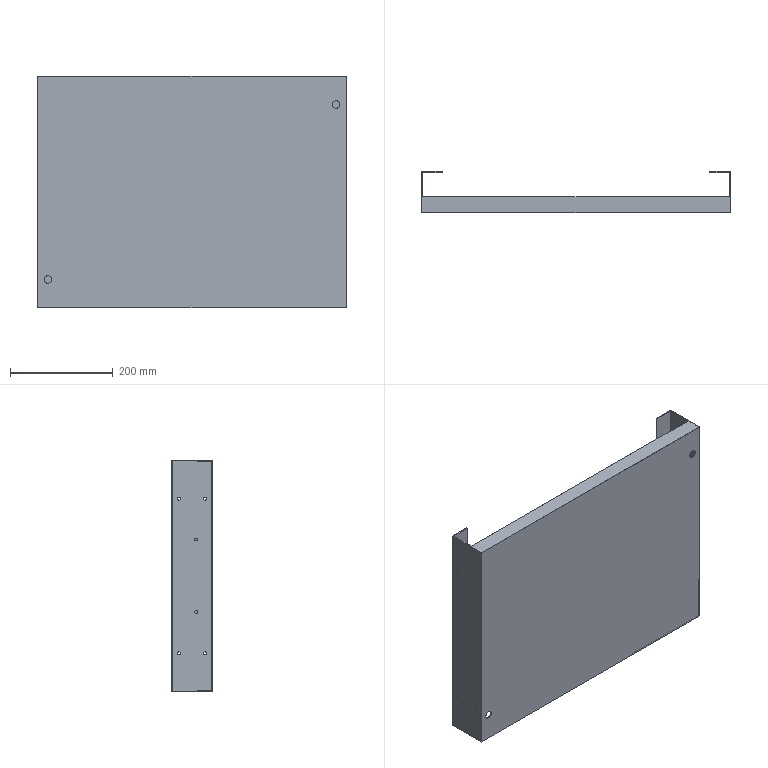Part | SolidWorks | features BaseBody 1 | 1 solid | 42 faces | box 600 x 80 x 450 mm | volume 814370 mm3 | cylinder 24 | plane 18 | commonest cylinder face diameters 5.5 x20 15 x4
STEP:
#1=CARTESIAN_POINT('',(301.946,-4083.973,1922.471));
#2=VERTEX_POINT('',#1);
#3=CARTESIAN_POINT('',(301.946,-4083.973,1907.471));
#4=VERTEX_POINT('',#3);
#5=CARTESIAN_POINT('',(301.946,-4083.973,1914.971));
#6=DIRECTION('',(0.,-1.,0.));
#7=DIRECTION('',(0.,0.,-1.));
#8=AXIS2_PLACEMENT_3D('',#5,#6,#7);
#9=CIRCLE('',#8,7.5);
#10=EDGE_CURVE('',#2,#4,#9,.T.);
#11=ORIENTED_EDGE('',*,*,#10,.F.);
#12=CARTESIAN_POINT('',(301.946,-4085.973,1922.471));
#13=VERTEX_POINT('',#12);
#14=CARTESIAN_POINT('',(301.946,-4104.978,1922.471));
#15=DIRECTION('',(0.,-1.,0.));
#16=VECTOR('',#15,1000.);
#17=LINE('',#14,#16);
#18=EDGE_CURVE('',#2,#13,#17,.T.);
#19=ORIENTED_EDGE('',*,*,#18,.T.);
#20=CARTESIAN_POINT('',(301.946,-4085.973,1907.471));
#21=VERTEX_POINT('',#20);
#22=CARTESIAN_POINT('',(301.946,-4085.973,1914.971));
#23=DIRECTION('',(0.,1.,0.));
#24=DIRECTION('',(0.,0.,-1.));
#25=AXIS2_PLACEMENT_3D('',#22,#23,#24);
#26=CIRCLE('',#25,7.5);
#27=EDGE_CURVE('',#21,#13,#26,.T.);
#28=ORIENTED_EDGE('',*,*,#27,.F.);
#29=CARTESIAN_POINT('',(301.946,-4104.978,1907.471));
#30=DIRECTION('',(0.,-1.,0.));
#31=VECTOR('',#30,1000.);
#32=LINE('',#29,#31);
#33=EDGE_CURVE('',#4,#21,#32,.T.);
#34=ORIENTED_EDGE('',*,*,#33,.F.);
#35=EDGE_LOOP('',(#11,#19,#28,#34));
#36=FACE_OUTER_BOUND('',#35,.T.);
#37=CARTESIAN_POINT('',(301.946,-4104.978,1914.971));
#38=DIRECTION('',(0.,-1.,0.));
#39=DIRECTION('',(0.,0.,-1.));
#40=AXIS2_PLACEMENT_3D('',#37,#38,#39);
#41=CYLINDRICAL_SURFACE('',#40,7.5);
#42=ADVANCED_FACE('',(#36),#41,.F.);
#43=CARTESIAN_POINT('',(861.946,-4083.973,2262.471));
#44=VERTEX_POINT('',#43);
#45=CARTESIAN_POINT('',(861.946,-4083.973,2247.471));
#46=VERTEX_POINT('',#45);
#47=CARTESIAN_POINT('',(861.946,-4083.973,2254.971));
#48=DIRECTION('',(0.,-1.,0.));
#49=DIRECTION('',(0.,0.,-1.));
#50=AXIS2_PLACEMENT_3D('',#47,#48,#49);
#51=CIRCLE('',#50,7.5);
#52=EDGE_CURVE('',#44,#46,#51,.T.);
#53=ORIENTED_EDGE('',*,*,#52,.F.);
#54=CARTESIAN_POINT('',(861.946,-4085.973,2262.471));
#55=VERTEX_POINT('',#54);
#56=CARTESIAN_POINT('',(861.946,-4082.758,2262.471));
#57=DIRECTION('',(0.,-1.,0.));
#58=VECTOR('',#57,1000.);
#59=LINE('',#56,#58);
#60=EDGE_CURVE('',#44,#55,#59,.T.);
#61=ORIENTED_EDGE('',*,*,#60,.T.);
#62=CARTESIAN_POINT('',(861.946,-4085.973,2247.471));
#63=VERTEX_POINT('',#62);
#64=CARTESIAN_POINT('',(861.946,-4085.973,2254.971));
#65=DIRECTION('',(0.,1.,0.));
#66=DIRECTION('',(0.,0.,-1.));
#67=AXIS2_PLACEMENT_3D('',#64,#65,#66);
#68=CIRCLE('',#67,7.5);
#69=EDGE_CURVE('',#63,#55,#68,.T.);
#70=ORIENTED_EDGE('',*,*,#69,.F.);
#71=CARTESIAN_POINT('',(861.946,-4082.758,2247.471));
#72=DIRECTION('',(0.,-1.,0.));
#73=VECTOR('',#72,1000.);
#74=LINE('',#71,#73);
#75=EDGE_CURVE('',#46,#63,#74,.T.);
#76=ORIENTED_EDGE('',*,*,#75,.F.);
#77=EDGE_LOOP('',(#53,#61,#70,#76));
#78=FACE_OUTER_BOUND('',#77,.T.);
#79=CARTESIAN_POINT('',(861.946,-4082.758,2254.971));
#80=DIRECTION('',(0.,-1.,0.));
#81=DIRECTION('',(0.,0.,-1.));
#82=AXIS2_PLACEMENT_3D('',#79,#80,#81);
#83=CYLINDRICAL_SURFACE('',#82,7.5);
#84=ADVANCED_FACE('',(#78),#83,.F.);
#85=CARTESIAN_POINT('',(283.946,-4053.971,2153.221));
#86=VERTEX_POINT('',#85);
#87=CARTESIAN_POINT('',(283.946,-4053.971,2158.721));
#88=VERTEX_POINT('',#87);
#89=CARTESIAN_POINT('',(283.946,-4053.971,2155.971));
#90=DIRECTION('',(-1.,0.,0.));
#91=DIRECTION('',(0.,0.,1.));
#92=AXIS2_PLACEMENT_3D('',#89,#90,#91);
#93=CIRCLE('',#92,2.75);
#94=EDGE_CURVE('',#86,#88,#93,.T.);
#95=ORIENTED_EDGE('',*,*,#94,.F.);
#96=CARTESIAN_POINT('',(281.946,-4053.971,2153.221));
#97=VERTEX_POINT('',#96);
#98=CARTESIAN_POINT('',(265.507,-4053.971,2153.221));
#99=DIRECTION('',(-1.,0.,0.));
#100=VECTOR('',#99,1000.);
#101=LINE('',#98,#100);
#102=EDGE_CURVE('',#86,#97,#101,.T.);
#103=ORIENTED_EDGE('',*,*,#102,.T.);
#104=CARTESIAN_POINT('',(281.946,-4053.971,2158.721));
#105=VERTEX_POINT('',#104);
#106=CARTESIAN_POINT('',(281.946,-4053.971,2155.971));
#107=DIRECTION('',(1.,0.,0.));
#108=DIRECTION('',(0.,0.,1.));
#109=AXIS2_PLACEMENT_3D('',#106,#107,#108);
#110=CIRCLE('',#109,2.75);
#111=EDGE_CURVE('',#105,#97,#110,.T.);
#112=ORIENTED_EDGE('',*,*,#111,.F.);
#113=CARTESIAN_POINT('',(265.507,-4053.971,2158.721));
#114=DIRECTION('',(-1.,0.,0.));
#115=VECTOR('',#114,1000.);
#116=LINE('',#113,#115);
#117=EDGE_CURVE('',#88,#105,#116,.T.);
#118=ORIENTED_EDGE('',*,*,#117,.F.);
#119=EDGE_LOOP('',(#95,#103,#112,#118));
#120=FACE_OUTER_BOUND('',#119,.T.);
#121=CARTESIAN_POINT('',(265.507,-4053.971,2155.971));
#122=DIRECTION('',(-1.,0.,0.));
#123=DIRECTION('',(0.,0.,1.));
#124=AXIS2_PLACEMENT_3D('',#121,#122,#123);
#125=CYLINDRICAL_SURFACE('',#124,2.75);
#126=ADVANCED_FACE('',(#120),#125,.F.);
#127=CARTESIAN_POINT('',(283.946,-4053.971,2012.221));
#128=VERTEX_POINT('',#127);
#129=CARTESIAN_POINT('',(283.946,-4053.971,2017.721));
#130=VERTEX_POINT('',#129);
#131=CARTESIAN_POINT('',(283.946,-4053.971,2014.971));
#132=DIRECTION('',(-1.,0.,0.));
#133=DIRECTION('',(0.,0.,1.));
#134=AXIS2_PLACEMENT_3D('',#131,#132,#133);
#135=CIRCLE('',#134,2.75);
#136=EDGE_CURVE('',#128,#130,#135,.T.);
#137=ORIENTED_EDGE('',*,*,#136,.F.);
#138=CARTESIAN_POINT('',(281.946,-4053.971,2012.221));
#139=VERTEX_POINT('',#138);
#140=CARTESIAN_POINT('',(265.507,-4053.971,2012.221));
#141=DIRECTION('',(-1.,0.,0.));
#142=VECTOR('',#141,1000.);
#143=LINE('',#140,#142);
#144=EDGE_CURVE('',#128,#139,#143,.T.);
#145=ORIENTED_EDGE('',*,*,#144,.T.);
#146=CARTESIAN_POINT('',(281.946,-4053.971,2017.721));
#147=VERTEX_POINT('',#146);
#148=CARTESIAN_POINT('',(281.946,-4053.971,2014.971));
#149=DIRECTION('',(1.,0.,0.));
#150=DIRECTION('',(0.,0.,1.));
#151=AXIS2_PLACEMENT_3D('',#148,#149,#150);
#152=CIRCLE('',#151,2.75);
#153=EDGE_CURVE('',#147,#139,#152,.T.);
#154=ORIENTED_EDGE('',*,*,#153,.F.);
#155=CARTESIAN_POINT('',(265.507,-4053.971,2017.721));
#156=DIRECTION('',(-1.,0.,0.));
#157=VECTOR('',#156,1000.);
#158=LINE('',#155,#157);
#159=EDGE_CURVE('',#130,#147,#158,.T.);
#160=ORIENTED_EDGE('',*,*,#159,.F.);
#161=EDGE_LOOP('',(#137,#145,#154,#160));
#162=FACE_OUTER_BOUND('',#161,.T.);
#163=CARTESIAN_POINT('',(265.507,-4053.971,2014.971));
#164=DIRECTION('',(-1.,0.,0.));
#165=DIRECTION('',(0.,0.,1.));
#166=AXIS2_PLACEMENT_3D('',#163,#164,#165);
#167=CYLINDRICAL_SURFACE('',#166,2.75);
#168=ADVANCED_FACE('',(#162),#167,.F.);
#169=CARTESIAN_POINT('',(283.946,-4020.973,2232.221));
#170=VERTEX_POINT('',#169);
#171=CARTESIAN_POINT('',(283.946,-4020.973,2237.721));
#172=VERTEX_POINT('',#171);
#173=CARTESIAN_POINT('',(283.946,-4020.973,2234.971));
#174=DIRECTION('',(-1.,0.,0.));
#175=DIRECTION('',(0.,0.,1.));
#176=AXIS2_PLACEMENT_3D('',#173,#174,#175);
#177=CIRCLE('',#176,2.75);
#178=EDGE_CURVE('',#170,#172,#177,.T.);
#179=ORIENTED_EDGE('',*,*,#178,.F.);
#180=CARTESIAN_POINT('',(281.946,-4020.973,2232.221));
#181=VERTEX_POINT('',#180);
#182=CARTESIAN_POINT('',(284.252,-4020.973,2232.221));
#183=DIRECTION('',(-1.,0.,0.));
#184=VECTOR('',#183,1000.);
#185=LINE('',#182,#184);
#186=EDGE_CURVE('',#170,#181,#185,.T.);
#187=ORIENTED_EDGE('',*,*,#186,.T.);
#188=CARTESIAN_POINT('',(281.946,-4020.973,2237.721));
#189=VERTEX_POINT('',#188);
#190=CARTESIAN_POINT('',(281.946,-4020.973,2234.971));
#191=DIRECTION('',(1.,0.,0.));
#192=DIRECTION('',(0.,0.,1.));
#193=AXIS2_PLACEMENT_3D('',#190,#191,#192);
#194=CIRCLE('',#193,2.75);
#195=EDGE_CURVE('',#189,#181,#194,.T.);
#196=ORIENTED_EDGE('',*,*,#195,.F.);
#197=CARTESIAN_POINT('',(284.252,-4020.973,2237.721));
#198=DIRECTION('',(-1.,0.,0.));
#199=VECTOR('',#198,1000.);
#200=LINE('',#197,#199);
#201=EDGE_CURVE('',#172,#189,#200,.T.);
#202=ORIENTED_EDGE('',*,*,#201,.F.);
#203=EDGE_LOOP('',(#179,#187,#196,#202));
#204=FACE_OUTER_BOUND('',#203,.T.);
#205=CARTESIAN_POINT('',(284.252,-4020.973,2234.971));
#206=DIRECTION('',(-1.,0.,0.));
#207=DIRECTION('',(0.,0.,1.));
#208=AXIS2_PLACEMENT_3D('',#205,#206,#207);
#209=CYLINDRICAL_SURFACE('',#208,2.75);
#210=ADVANCED_FACE('',(#204),#209,.F.);
#211=CARTESIAN_POINT('',(283.946,-4070.973,2232.221));
#212=VERTEX_POINT('',#211);
#213=CARTESIAN_POINT('',(283.946,-4070.973,2237.721));
#214=VERTEX_POINT('',#213);
#215=CARTESIAN_POINT('',(283.946,-4070.973,2234.971));
#216=DIRECTION('',(-1.,0.,0.));
#217=DIRECTION('',(0.,0.,1.));
#218=AXIS2_PLACEMENT_3D('',#215,#216,#217);
#219=CIRCLE('',#218,2.75);
#220=EDGE_CURVE('',#212,#214,#219,.T.);
#221=ORIENTED_EDGE('',*,*,#220,.F.);
#222=CARTESIAN_POINT('',(281.946,-4070.973,2232.221));
#223=VERTEX_POINT('',#222);
#224=CARTESIAN_POINT('',(284.252,-4070.973,2232.221));
#225=DIRECTION('',(-1.,0.,0.));
#226=VECTOR('',#225,1000.);
#227=LINE('',#224,#226);
#228=EDGE_CURVE('',#212,#223,#227,.T.);
#229=ORIENTED_EDGE('',*,*,#228,.T.);
#230=CARTESIAN_POINT('',(281.946,-4070.973,2237.721));
#231=VERTEX_POINT('',#230);
#232=CARTESIAN_POINT('',(281.946,-4070.973,2234.971));
#233=DIRECTION('',(1.,0.,0.));
#234=DIRECTION('',(0.,0.,1.));
#235=AXIS2_PLACEMENT_3D('',#232,#233,#234);
#236=CIRCLE('',#235,2.75);
#237=EDGE_CURVE('',#231,#223,#236,.T.);
#238=ORIENTED_EDGE('',*,*,#237,.F.);
#239=CARTESIAN_POINT('',(284.252,-4070.973,2237.721));
#240=DIRECTION('',(-1.,0.,0.));
#241=VECTOR('',#240,1000.);
#242=LINE('',#239,#241);
#243=EDGE_CURVE('',#214,#231,#242,.T.);
#244=ORIENTED_EDGE('',*,*,#243,.F.);
#245=EDGE_LOOP('',(#221,#229,#238,#244));
#246=FACE_OUTER_BOUND('',#245,.T.);
#247=CARTESIAN_POINT('',(284.252,-4070.973,2234.971));
#248=DIRECTION('',(-1.,0.,0.));
#249=DIRECTION('',(0.,0.,1.));
#250=AXIS2_PLACEMENT_3D('',#247,#248,#249);
#251=CYLINDRICAL_SURFACE('',#250,2.75);
#252=ADVANCED_FACE('',(#246),#251,.F.);
#253=CARTESIAN_POINT('',(281.946,-4070.973,1937.721));
#254=VERTEX_POINT('',#253);
#255=CARTESIAN_POINT('',(281.946,-4070.973,1932.221));
#256=VERTEX_POINT('',#255);
#257=CARTESIAN_POINT('',(281.946,-4070.973,1934.971));
#258=DIRECTION('',(1.,0.,0.));
#259=DIRECTION('',(0.,0.,-1.));
#260=AXIS2_PLACEMENT_3D('',#257,#258,#259);
#261=CIRCLE('',#260,2.75);
#262=EDGE_CURVE('',#254,#256,#261,.T.);
#263=ORIENTED_EDGE('',*,*,#262,.F.);
#264=CARTESIAN_POINT('',(283.946,-4070.973,1937.721));
#265=VERTEX_POINT('',#264);
#266=CARTESIAN_POINT('',(284.252,-4070.973,1937.721));
#267=DIRECTION('',(1.,0.,0.));
#268=VECTOR('',#267,1000.);
#269=LINE('',#266,#268);
#270=EDGE_CURVE('',#254,#265,#269,.T.);
#271=ORIENTED_EDGE('',*,*,#270,.T.);
#272=CARTESIAN_POINT('',(283.946,-4070.973,1932.221));
#273=VERTEX_POINT('',#272);
#274=CARTESIAN_POINT('',(283.946,-4070.973,1934.971));
#275=DIRECTION('',(-1.,0.,0.));
#276=DIRECTION('',(0.,0.,-1.));
#277=AXIS2_PLACEMENT_3D('',#274,#275,#276);
#278=CIRCLE('',#277,2.75);
#279=EDGE_CURVE('',#273,#265,#278,.T.);
#280=ORIENTED_EDGE('',*,*,#279,.F.);
#281=CARTESIAN_POINT('',(284.252,-4070.973,1932.221));
#282=DIRECTION('',(1.,0.,0.));
#283=VECTOR('',#282,1000.);
#284=LINE('',#281,#283);
#285=EDGE_CURVE('',#256,#273,#284,.T.);
#286=ORIENTED_EDGE('',*,*,#285,.F.);
#287=EDGE_LOOP('',(#263,#271,#280,#286));
#288=FACE_OUTER_BOUND('',#287,.T.);
#289=CARTESIAN_POINT('',(284.252,-4070.973,1934.971));
#290=DIRECTION('',(1.,0.,0.));
#291=DIRECTION('',(0.,0.,-1.));
#292=AXIS2_PLACEMENT_3D('',#289,#290,#291);
#293=CYLINDRICAL_SURFACE('',#292,2.75);
#294=ADVANCED_FACE('',(#288),#293,.F.);
#295=CARTESIAN_POINT('',(281.946,-4020.973,1937.721));
#296=VERTEX_POINT('',#295);
#297=CARTESIAN_POINT('',(281.946,-4020.973,1932.221));
#298=VERTEX_POINT('',#297);
#299=CARTESIAN_POINT('',(281.946,-4020.973,1934.971));
#300=DIRECTION('',(1.,0.,0.));
#301=DIRECTION('',(0.,0.,-1.));
#302=AXIS2_PLACEMENT_3D('',#299,#300,#301);
#303=CIRCLE('',#302,2.75);
#304=EDGE_CURVE('',#296,#298,#303,.T.);
#305=ORIENTED_EDGE('',*,*,#304,.F.);
#306=CARTESIAN_POINT('',(283.946,-4020.973,1937.721));
#307=VERTEX_POINT('',#306);
#308=CARTESIAN_POINT('',(284.252,-4020.973,1937.721));
#309=DIRECTION('',(1.,0.,0.));
#310=VECTOR('',#309,1000.);
#311=LINE('',#308,#310);
#312=EDGE_CURVE('',#296,#307,#311,.T.);
#313=ORIENTED_EDGE('',*,*,#312,.T.);
#314=CARTESIAN_POINT('',(283.946,-4020.973,1932.221));
#315=VERTEX_POINT('',#314);
#316=CARTESIAN_POINT('',(283.946,-4020.973,1934.971));
#317=DIRECTION('',(-1.,0.,0.));
#318=DIRECTION('',(0.,0.,-1.));
#319=AXIS2_PLACEMENT_3D('',#316,#317,#318);
#320=CIRCLE('',#319,2.75);
#321=EDGE_CURVE('',#315,#307,#320,.T.);
#322=ORIENTED_EDGE('',*,*,#321,.F.);
#323=CARTESIAN_POINT('',(284.252,-4020.973,1932.221));
#324=DIRECTION('',(1.,0.,0.));
#325=VECTOR('',#324,1000.);
#326=LINE('',#323,#325);
#327=EDGE_CURVE('',#298,#315,#326,.T.);
#328=ORIENTED_EDGE('',*,*,#327,.F.);
#329=EDGE_LOOP('',(#305,#313,#322,#328));
#330=FACE_OUTER_BOUND('',#329,.T.);
#331=CARTESIAN_POINT('',(284.252,-4020.973,1934.971));
#332=DIRECTION('',(1.,0.,0.));
#333=DIRECTION('',(0.,0.,-1.));
#334=AXIS2_PLACEMENT_3D('',#331,#332,#333);
#335=CYLINDRICAL_SURFACE('',#334,2.75);
#336=ADVANCED_FACE('',(#330),#335,.F.);
#337=CARTESIAN_POINT('',(881.946,-4070.973,2232.221));
#338=VERTEX_POINT('',#337);
#339=CARTESIAN_POINT('',(881.946,-4070.973,2237.721));
#340=VERTEX_POINT('',#339);
#341=CARTESIAN_POINT('',(881.946,-4070.973,2234.971));
#342=DIRECTION('',(-1.,0.,0.));
#343=DIRECTION('',(0.,0.,1.));
#344=AXIS2_PLACEMENT_3D('',#341,#342,#343);
#345=CIRCLE('',#344,2.75);
#346=EDGE_CURVE('',#338,#340,#345,.T.);
#347=ORIENTED_EDGE('',*,*,#346,.F.);
#348=CARTESIAN_POINT('',(879.946,-4070.973,2232.221));
#349=VERTEX_POINT('',#348);
#350=CARTESIAN_POINT('',(879.639,-4070.973,2232.221));
#351=DIRECTION('',(-1.,0.,0.));
#352=VECTOR('',#351,1000.);
#353=LINE('',#350,#352);
#354=EDGE_CURVE('',#338,#349,#353,.T.);
#355=ORIENTED_EDGE('',*,*,#354,.T.);
#356=CARTESIAN_POINT('',(879.946,-4070.973,2237.721));
#357=VERTEX_POINT('',#356);
#358=CARTESIAN_POINT('',(879.946,-4070.973,2234.971));
#359=DIRECTION('',(1.,0.,0.));
#360=DIRECTION('',(0.,0.,1.));
#361=AXIS2_PLACEMENT_3D('',#358,#359,#360);
#362=CIRCLE('',#361,2.75);
#363=EDGE_CURVE('',#357,#349,#362,.T.);
#364=ORIENTED_EDGE('',*,*,#363,.F.);
#365=CARTESIAN_POINT('',(879.639,-4070.973,2237.721));
#366=DIRECTION('',(-1.,0.,0.));
#367=VECTOR('',#366,1000.);
#368=LINE('',#365,#367);
#369=EDGE_CURVE('',#340,#357,#368,.T.);
#370=ORIENTED_EDGE('',*,*,#369,.F.);
#371=EDGE_LOOP('',(#347,#355,#364,#370));
#372=FACE_OUTER_BOUND('',#371,.T.);
#373=CARTESIAN_POINT('',(879.639,-4070.973,2234.971));
#374=DIRECTION('',(-1.,0.,0.));
#375=DIRECTION('',(0.,0.,1.));
#376=AXIS2_PLACEMENT_3D('',#373,#374,#375);
#377=CYLINDRICAL_SURFACE('',#376,2.75);
#378=ADVANCED_FACE('',(#372),#377,.F.);
#379=CARTESIAN_POINT('',(881.946,-4020.973,2232.221));
#380=VERTEX_POINT('',#379);
#381=CARTESIAN_POINT('',(881.946,-4020.973,2237.721));
#382=VERTEX_POINT('',#381);
#383=CARTESIAN_POINT('',(881.946,-4020.973,2234.971));
#384=DIRECTION('',(-1.,0.,0.));
#385=DIRECTION('',(0.,0.,1.));
#386=AXIS2_PLACEMENT_3D('',#383,#384,#385);
#387=CIRCLE('',#386,2.75);
#388=EDGE_CURVE('',#380,#382,#387,.T.);
#389=ORIENTED_EDGE('',*,*,#388,.F.);
#390=CARTESIAN_POINT('',(879.946,-4020.973,2232.221));
#391=VERTEX_POINT('',#390);
#392=CARTESIAN_POINT('',(879.639,-4020.973,2232.221));
#393=DIRECTION('',(-1.,0.,0.));
#394=VECTOR('',#393,1000.);
#395=LINE('',#392,#394);
#396=EDGE_CURVE('',#380,#391,#395,.T.);
#397=ORIENTED_EDGE('',*,*,#396,.T.);
#398=CARTESIAN_POINT('',(879.946,-4020.973,2237.721));
#399=VERTEX_POINT('',#398);
#400=CARTESIAN_POINT('',(879.946,-4020.973,2234.971));
#401=DIRECTION('',(1.,0.,0.));
#402=DIRECTION('',(0.,0.,1.));
#403=AXIS2_PLACEMENT_3D('',#400,#401,#402);
#404=CIRCLE('',#403,2.75);
#405=EDGE_CURVE('',#399,#391,#404,.T.);
#406=ORIENTED_EDGE('',*,*,#405,.F.);
#407=CARTESIAN_POINT('',(879.639,-4020.973,2237.721));
#408=DIRECTION('',(-1.,0.,0.));
#409=VECTOR('',#408,1000.);
#410=LINE('',#407,#409);
#411=EDGE_CURVE('',#382,#399,#410,.T.);
#412=ORIENTED_EDGE('',*,*,#411,.F.);
#413=EDGE_LOOP('',(#389,#397,#406,#412));
#414=FACE_OUTER_BOUND('',#413,.T.);
#415=CARTESIAN_POINT('',(879.639,-4020.973,2234.971));
#416=DIRECTION('',(-1.,0.,0.));
#417=DIRECTION('',(0.,0.,1.));
#418=AXIS2_PLACEMENT_3D('',#415,#416,#417);
#419=CYLINDRICAL_SURFACE('',#418,2.75);
#420=ADVANCED_FACE('',(#414),#419,.F.);
#421=CARTESIAN_POINT('',(879.946,-4020.973,1937.721));
#422=VERTEX_POINT('',#421);
#423=CARTESIAN_POINT('',(879.946,-4020.973,1932.221));
#424=VERTEX_POINT('',#423);
#425=CARTESIAN_POINT('',(879.946,-4020.973,1934.971));
#426=DIRECTION('',(1.,0.,0.));
#427=DIRECTION('',(0.,0.,-1.));
#428=AXIS2_PLACEMENT_3D('',#425,#426,#427);
#429=CIRCLE('',#428,2.75);
#430=EDGE_CURVE('',#422,#424,#429,.T.);
#431=ORIENTED_EDGE('',*,*,#430,.F.);
#432=CARTESIAN_POINT('',(881.946,-4020.973,1937.721));
#433=VERTEX_POINT('',#432);
#434=CARTESIAN_POINT('',(879.639,-4020.973,1937.721));
#435=DIRECTION('',(1.,0.,0.));
#436=VECTOR('',#435,1000.);
#437=LINE('',#434,#436);
#438=EDGE_CURVE('',#422,#433,#437,.T.);
#439=ORIENTED_EDGE('',*,*,#438,.T.);
#440=CARTESIAN_POINT('',(881.946,-4020.973,1932.221));
#441=VERTEX_POINT('',#440);
#442=CARTESIAN_POINT('',(881.946,-4020.973,1934.971));
#443=DIRECTION('',(-1.,0.,0.));
#444=DIRECTION('',(0.,0.,-1.));
#445=AXIS2_PLACEMENT_3D('',#442,#443,#444);
#446=CIRCLE('',#445,2.75);
#447=EDGE_CURVE('',#441,#433,#446,.T.);
#448=ORIENTED_EDGE('',*,*,#447,.F.);
#449=CARTESIAN_POINT('',(879.639,-4020.973,1932.221));
#450=DIRECTION('',(1.,0.,0.));
#451=VECTOR('',#450,1000.);
#452=LINE('',#449,#451);
#453=EDGE_CURVE('',#424,#441,#452,.T.);
#454=ORIENTED_EDGE('',*,*,#453,.F.);
#455=EDGE_LOOP('',(#431,#439,#448,#454));
#456=FACE_OUTER_BOUND('',#455,.T.);
#457=CARTESIAN_POINT('',(879.639,-4020.973,1934.971));
#458=DIRECTION('',(1.,0.,0.));
#459=DIRECTION('',(0.,0.,-1.));
#460=AXIS2_PLACEMENT_3D('',#457,#458,#459);
#461=CYLINDRICAL_SURFACE('',#460,2.75);
#462=ADVANCED_FACE('',(#456),#461,.F.);
#463=CARTESIAN_POINT('',(879.946,-4070.973,1937.721));
#464=VERTEX_POINT('',#463);
#465=CARTESIAN_POINT('',(879.946,-4070.973,1932.221));
#466=VERTEX_POINT('',#465);
#467=CARTESIAN_POINT('',(879.946,-4070.973,1934.971));
#468=DIRECTION('',(1.,0.,0.));
#469=DIRECTION('',(0.,0.,-1.));
#470=AXIS2_PLACEMENT_3D('',#467,#468,#469);
#471=CIRCLE('',#470,2.75);
#472=EDGE_CURVE('',#464,#466,#471,.T.);
#473=ORIENTED_EDGE('',*,*,#472,.F.);
#474=CARTESIAN_POINT('',(881.946,-4070.973,1937.721));
#475=VERTEX_POINT('',#474);
#476=CARTESIAN_POINT('',(879.639,-4070.973,1937.721));
#477=DIRECTION('',(1.,0.,0.));
#478=VECTOR('',#477,1000.);
#479=LINE('',#476,#478);
#480=EDGE_CURVE('',#464,#475,#479,.T.);
#481=ORIENTED_EDGE('',*,*,#480,.T.);
#482=CARTESIAN_POINT('',(881.946,-4070.973,1932.221));
#483=VERTEX_POINT('',#482);
#484=CARTESIAN_POINT('',(881.946,-4070.973,1934.971));
#485=DIRECTION('',(-1.,0.,0.));
#486=DIRECTION('',(0.,0.,-1.));
#487=AXIS2_PLACEMENT_3D('',#484,#485,#486);
#488=CIRCLE('',#487,2.75);
#489=EDGE_CURVE('',#483,#475,#488,.T.);
#490=ORIENTED_EDGE('',*,*,#489,.F.);
#491=CARTESIAN_POINT('',(879.639,-4070.973,1932.221));
#492=DIRECTION('',(1.,0.,0.));
#493=VECTOR('',#492,1000.);
#494=LINE('',#491,#493);
#495=EDGE_CURVE('',#466,#483,#494,.T.);
#496=ORIENTED_EDGE('',*,*,#495,.F.);
#497=EDGE_LOOP('',(#473,#481,#490,#496));
#498=FACE_OUTER_BOUND('',#497,.T.);
#499=CARTESIAN_POINT('',(879.639,-4070.973,1934.971));
#500=DIRECTION('',(1.,0.,0.));
#501=DIRECTION('',(0.,0.,-1.));
#502=AXIS2_PLACEMENT_3D('',#499,#500,#501);
#503=CYLINDRICAL_SURFACE('',#502,2.75);
#504=ADVANCED_FACE('',(#498),#503,.F.);
#505=CARTESIAN_POINT('',(281.946,-4085.973,2309.971));
#506=VERTEX_POINT('',#505);
#507=CARTESIAN_POINT('',(281.946,-4085.973,1859.971));
#508=VERTEX_POINT('',#507);
#509=CARTESIAN_POINT('',(281.946,-4085.973,2309.971));
#510=DIRECTION('',(0.,0.,-1.));
#511=VECTOR('',#510,1000.);
#512=LINE('',#509,#511);
#513=EDGE_CURVE('',#506,#508,#512,.T.);
#514=ORIENTED_EDGE('',*,*,#513,.T.);
#515=CARTESIAN_POINT('',(881.946,-4085.973,1859.971));
#516=VERTEX_POINT('',#515);
#517=CARTESIAN_POINT('',(881.946,-4085.973,1859.971));
#518=DIRECTION('',(1.,0.,0.));
#519=VECTOR('',#518,1000.);
#520=LINE('',#517,#519);
#521=EDGE_CURVE('',#508,#516,#520,.T.);
#522=ORIENTED_EDGE('',*,*,#521,.T.);
#523=CARTESIAN_POINT('',(881.946,-4085.973,2309.971));
#524=VERTEX_POINT('',#523);
#525=CARTESIAN_POINT('',(881.946,-4085.973,2309.971));
#526=DIRECTION('',(0.,0.,1.));
#527=VECTOR('',#526,1000.);
#528=LINE('',#525,#527);
#529=EDGE_CURVE('',#516,#524,#528,.T.);
#530=ORIENTED_EDGE('',*,*,#529,.T.);
#531=CARTESIAN_POINT('',(881.946,-4085.973,2309.971));
#532=DIRECTION('',(-1.,0.,0.));
#533=VECTOR('',#532,1000.);
#534=LINE('',#531,#533);
#535=EDGE_CURVE('',#524,#506,#534,.T.);
#536=ORIENTED_EDGE('',*,*,#535,.T.);
#537=EDGE_LOOP('',(#514,#522,#530,#536));
#538=FACE_OUTER_BOUND('',#537,.T.);
#539=ORIENTED_EDGE('',*,*,#27,.T.);
#540=CARTESIAN_POINT('',(301.946,-4085.973,1914.971));
#541=DIRECTION('',(0.,1.,0.));
#542=DIRECTION('',(0.,0.,-1.));
#543=AXIS2_PLACEMENT_3D('',#540,#541,#542);
#544=CIRCLE('',#543,7.5);
#545=EDGE_CURVE('',#13,#21,#544,.T.);
#546=ORIENTED_EDGE('',*,*,#545,.T.);
#547=EDGE_LOOP('',(#539,#546));
#548=FACE_BOUND('',#547,.T.);
#549=ORIENTED_EDGE('',*,*,#69,.T.);
#550=CARTESIAN_POINT('',(861.946,-4085.973,2254.971));
#551=DIRECTION('',(0.,1.,0.));
#552=DIRECTION('',(0.,0.,-1.));
#553=AXIS2_PLACEMENT_3D('',#550,#551,#552);
#554=CIRCLE('',#553,7.5);
#555=EDGE_CURVE('',#55,#63,#554,.T.);
#556=ORIENTED_EDGE('',*,*,#555,.T.);
#557=EDGE_LOOP('',(#549,#556));
#558=FACE_BOUND('',#557,.T.);
#559=CARTESIAN_POINT('',(881.946,-4085.973,2309.971));
#560=DIRECTION('',(0.,-1.,0.));
#561=DIRECTION('',(0.,0.,-1.));
#562=AXIS2_PLACEMENT_3D('',#559,#560,#561);
#563=PLANE('',#562);
#564=ADVANCED_FACE('',(#538,#548,#558),#563,.T.);
#565=CARTESIAN_POINT('',(879.946,-4007.973,1859.971));
#566=VERTEX_POINT('',#565);
#567=CARTESIAN_POINT('',(879.946,-4055.973,1859.971));
#568=VERTEX_POINT('',#567);
#569=CARTESIAN_POINT('',(879.946,-4070.973,1859.971));
#570=DIRECTION('',(0.,-1.,0.));
#571=VECTOR('',#570,1000.);
#572=LINE('',#569,#571);
#573=EDGE_CURVE('',#566,#568,#572,.T.);
#574=ORIENTED_EDGE('',*,*,#573,.F.);
#575=CARTESIAN_POINT('',(841.946,-4007.973,1859.971));
#576=VERTEX_POINT('',#575);
#577=CARTESIAN_POINT('',(581.946,-4007.973,1859.971));
#578=DIRECTION('',(1.,0.,0.));
#579=VECTOR('',#578,1000.);
#580=LINE('',#577,#579);
#581=EDGE_CURVE('',#576,#566,#580,.T.);
#582=ORIENTED_EDGE('',*,*,#581,.F.);
#583=CARTESIAN_POINT('',(841.946,-4005.973,1859.971));
#584=VERTEX_POINT('',#583);
#585=CARTESIAN_POINT('',(841.946,-4070.973,1859.971));
#586=DIRECTION('',(0.,-1.,0.));
#587=VECTOR('',#586,1000.);
#588=LINE('',#585,#587);
#589=EDGE_CURVE('',#584,#576,#588,.T.);
#590=ORIENTED_EDGE('',*,*,#589,.F.);
#591=CARTESIAN_POINT('',(881.946,-4005.973,1859.971));
#592=VERTEX_POINT('',#591);
#593=CARTESIAN_POINT('',(581.946,-4005.973,1859.971));
#594=DIRECTION('',(-1.,0.,0.));
#595=VECTOR('',#594,1000.);
#596=LINE('',#593,#595);
#597=EDGE_CURVE('',#592,#584,#596,.T.);
#598=ORIENTED_EDGE('',*,*,#597,.F.);
#599=CARTESIAN_POINT('',(881.946,-4070.973,1859.971));
#600=DIRECTION('',(0.,1.,0.));
#601=VECTOR('',#600,1000.);
#602=LINE('',#599,#601);
#603=EDGE_CURVE('',#516,#592,#602,.T.);
#604=ORIENTED_EDGE('',*,*,#603,.F.);
#605=ORIENTED_EDGE('',*,*,#521,.F.);
#606=CARTESIAN_POINT('',(281.946,-4005.973,1859.971));
#607=VERTEX_POINT('',#606);
#608=CARTESIAN_POINT('',(281.946,-4070.973,1859.971));
#609=DIRECTION('',(0.,-1.,0.));
#610=VECTOR('',#609,1000.);
#611=LINE('',#608,#610);
#612=EDGE_CURVE('',#607,#508,#611,.T.);
#613=ORIENTED_EDGE('',*,*,#612,.F.);
#614=CARTESIAN_POINT('',(321.946,-4005.973,1859.971));
#615=VERTEX_POINT('',#614);
#616=CARTESIAN_POINT('',(581.946,-4005.973,1859.971));
#617=DIRECTION('',(-1.,0.,0.));
#618=VECTOR('',#617,1000.);
#619=LINE('',#616,#618);
#620=EDGE_CURVE('',#615,#607,#619,.T.);
#621=ORIENTED_EDGE('',*,*,#620,.F.);
#622=CARTESIAN_POINT('',(321.946,-4007.973,1859.971));
#623=VERTEX_POINT('',#622);
#624=CARTESIAN_POINT('',(321.946,-4070.973,1859.971));
#625=DIRECTION('',(0.,1.,0.));
#626=VECTOR('',#625,1000.);
#627=LINE('',#624,#626);
#628=EDGE_CURVE('',#623,#615,#627,.T.);
#629=ORIENTED_EDGE('',*,*,#628,.F.);
#630=CARTESIAN_POINT('',(283.946,-4007.973,1859.971));
#631=VERTEX_POINT('',#630);
#632=CARTESIAN_POINT('',(581.946,-4007.973,1859.971));
#633=DIRECTION('',(1.,0.,0.));
#634=VECTOR('',#633,1000.);
#635=LINE('',#632,#634);
#636=EDGE_CURVE('',#631,#623,#635,.T.);
#637=ORIENTED_EDGE('',*,*,#636,.F.);
#638=CARTESIAN_POINT('',(283.946,-4055.973,1859.971));
#639=VERTEX_POINT('',#638);
#640=CARTESIAN_POINT('',(283.946,-4070.973,1859.971));
#641=DIRECTION('',(0.,1.,0.));
#642=VECTOR('',#641,1000.);
#643=LINE('',#640,#642);
#644=EDGE_CURVE('',#639,#631,#643,.T.);
#645=ORIENTED_EDGE('',*,*,#644,.F.);
#646=CARTESIAN_POINT('',(581.946,-4055.973,1859.971));
#647=DIRECTION('',(-1.,0.,0.));
#648=VECTOR('',#647,1000.);
#649=LINE('',#646,#648);
#650=EDGE_CURVE('',#568,#639,#649,.T.);
#651=ORIENTED_EDGE('',*,*,#650,.F.);
#652=EDGE_LOOP('',(#574,#582,#590,#598,#604,#605,#613,#621,#629,#637,#645,#651));
#653=FACE_OUTER_BOUND('',#652,.T.);
#654=CARTESIAN_POINT('',(581.946,-4070.973,1859.971));
#655=DIRECTION('',(0.,0.,1.));
#656=DIRECTION('',(1.,0.,0.));
#657=AXIS2_PLACEMENT_3D('',#654,#655,#656);
#658=PLANE('',#657);
#659=ADVANCED_FACE('',(#653),#658,.F.);
#660=CARTESIAN_POINT('',(281.946,-4005.973,2309.971));
#661=VERTEX_POINT('',#660);
#662=CARTESIAN_POINT('',(281.946,-4005.973,2309.971));
#663=DIRECTION('',(0.,0.,-1.));
#664=VECTOR('',#663,1000.);
#665=LINE('',#662,#664);
#666=EDGE_CURVE('',#661,#607,#665,.T.);
#667=ORIENTED_EDGE('',*,*,#666,.T.);
#668=ORIENTED_EDGE('',*,*,#612,.T.);
#669=ORIENTED_EDGE('',*,*,#513,.F.);
#670=CARTESIAN_POINT('',(281.946,-4085.973,2309.971));
#671=DIRECTION('',(0.,1.,0.));
#672=VECTOR('',#671,1000.);
#673=LINE('',#670,#672);
#674=EDGE_CURVE('',#506,#661,#673,.T.);
#675=ORIENTED_EDGE('',*,*,#674,.T.);
#676=EDGE_LOOP('',(#667,#668,#669,#675));
#677=FACE_OUTER_BOUND('',#676,.T.);
#678=ORIENTED_EDGE('',*,*,#111,.T.);
#679=CARTESIAN_POINT('',(281.946,-4053.971,2155.971));
#680=DIRECTION('',(1.,0.,0.));
#681=DIRECTION('',(0.,0.,1.));
#682=AXIS2_PLACEMENT_3D('',#679,#680,#681);
#683=CIRCLE('',#682,2.75);
#684=EDGE_CURVE('',#97,#105,#683,.T.);
#685=ORIENTED_EDGE('',*,*,#684,.T.);
#686=EDGE_LOOP('',(#678,#685));
#687=FACE_BOUND('',#686,.T.);
#688=ORIENTED_EDGE('',*,*,#153,.T.);
#689=CARTESIAN_POINT('',(281.946,-4053.971,2014.971));
#690=DIRECTION('',(1.,0.,0.));
#691=DIRECTION('',(0.,0.,1.));
#692=AXIS2_PLACEMENT_3D('',#689,#690,#691);
#693=CIRCLE('',#692,2.75);
#694=EDGE_CURVE('',#139,#147,#693,.T.);
#695=ORIENTED_EDGE('',*,*,#694,.T.);
#696=EDGE_LOOP('',(#688,#695));
#697=FACE_BOUND('',#696,.T.);
#698=ORIENTED_EDGE('',*,*,#195,.T.);
#699=CARTESIAN_POINT('',(281.946,-4020.973,2234.971));
#700=DIRECTION('',(1.,0.,0.));
#701=DIRECTION('',(0.,0.,1.));
#702=AXIS2_PLACEMENT_3D('',#699,#700,#701);
#703=CIRCLE('',#702,2.75);
#704=EDGE_CURVE('',#181,#189,#703,.T.);
#705=ORIENTED_EDGE('',*,*,#704,.T.);
#706=EDGE_LOOP('',(#698,#705));
#707=FACE_BOUND('',#706,.T.);
#708=ORIENTED_EDGE('',*,*,#237,.T.);
#709=CARTESIAN_POINT('',(281.946,-4070.973,2234.971));
#710=DIRECTION('',(1.,0.,0.));
#711=DIRECTION('',(0.,0.,1.));
#712=AXIS2_PLACEMENT_3D('',#709,#710,#711);
#713=CIRCLE('',#712,2.75);
#714=EDGE_CURVE('',#223,#231,#713,.T.);
#715=ORIENTED_EDGE('',*,*,#714,.T.);
#716=EDGE_LOOP('',(#708,#715));
#717=FACE_BOUND('',#716,.T.);
#718=CARTESIAN_POINT('',(281.946,-4070.973,1934.971));
#719=DIRECTION('',(1.,0.,0.));
#720=DIRECTION('',(0.,0.,-1.));
#721=AXIS2_PLACEMENT_3D('',#718,#719,#720);
#722=CIRCLE('',#721,2.75);
#723=EDGE_CURVE('',#256,#254,#722,.T.);
#724=ORIENTED_EDGE('',*,*,#723,.T.);
#725=ORIENTED_EDGE('',*,*,#262,.T.);
#726=EDGE_LOOP('',(#724,#725));
#727=FACE_BOUND('',#726,.T.);
#728=CARTESIAN_POINT('',(281.946,-4020.973,1934.971));
#729=DIRECTION('',(1.,0.,0.));
#730=DIRECTION('',(0.,0.,-1.));
#731=AXIS2_PLACEMENT_3D('',#728,#729,#730);
#732=CIRCLE('',#731,2.75);
#733=EDGE_CURVE('',#298,#296,#732,.T.);
#734=ORIENTED_EDGE('',*,*,#733,.T.);
#735=ORIENTED_EDGE('',*,*,#304,.T.);
#736=EDGE_LOOP('',(#734,#735));
#737=FACE_BOUND('',#736,.T.);
#738=CARTESIAN_POINT('',(281.946,-4085.973,2309.971));
#739=DIRECTION('',(-1.,0.,0.));
#740=DIRECTION('',(0.,0.,1.));
#741=AXIS2_PLACEMENT_3D('',#738,#739,#740);
#742=PLANE('',#741);
#743=ADVANCED_FACE('',(#677,#687,#697,#707,#717,#727,#737),#742,.T.);
#744=ORIENTED_EDGE('',*,*,#535,.F.);
#745=CARTESIAN_POINT('',(881.946,-4005.973,2309.971));
#746=VERTEX_POINT('',#745);
#747=CARTESIAN_POINT('',(881.946,-4070.973,2309.971));
#748=DIRECTION('',(0.,-1.,0.));
#749=VECTOR('',#748,1000.);
#750=LINE('',#747,#749);
#751=EDGE_CURVE('',#746,#524,#750,.T.);
#752=ORIENTED_EDGE('',*,*,#751,.F.);
#753=CARTESIAN_POINT('',(841.946,-4005.973,2309.971));
#754=VERTEX_POINT('',#753);
#755=CARTESIAN_POINT('',(581.946,-4005.973,2309.971));
#756=DIRECTION('',(1.,0.,0.));
#757=VECTOR('',#756,1000.);
#758=LINE('',#755,#757);
#759=EDGE_CURVE('',#754,#746,#758,.T.);
#760=ORIENTED_EDGE('',*,*,#759,.F.);
#761=CARTESIAN_POINT('',(841.946,-4007.973,2309.971));
#762=VERTEX_POINT('',#761);
#763=CARTESIAN_POINT('',(841.946,-4070.973,2309.971));
#764=DIRECTION('',(0.,1.,0.));
#765=VECTOR('',#764,1000.);
#766=LINE('',#763,#765);
#767=EDGE_CURVE('',#762,#754,#766,.T.);
#768=ORIENTED_EDGE('',*,*,#767,.F.);
#769=CARTESIAN_POINT('',(879.946,-4007.973,2309.971));
#770=VERTEX_POINT('',#769);
#771=CARTESIAN_POINT('',(581.946,-4007.973,2309.971));
#772=DIRECTION('',(-1.,0.,0.));
#773=VECTOR('',#772,1000.);
#774=LINE('',#771,#773);
#775=EDGE_CURVE('',#770,#762,#774,.T.);
#776=ORIENTED_EDGE('',*,*,#775,.F.);
#777=CARTESIAN_POINT('',(879.946,-4055.973,2309.971));
#778=VERTEX_POINT('',#777);
#779=CARTESIAN_POINT('',(879.946,-4070.973,2309.971));
#780=DIRECTION('',(0.,1.,0.));
#781=VECTOR('',#780,1000.);
#782=LINE('',#779,#781);
#783=EDGE_CURVE('',#778,#770,#782,.T.);
#784=ORIENTED_EDGE('',*,*,#783,.F.);
#785=CARTESIAN_POINT('',(283.946,-4055.973,2309.971));
#786=VERTEX_POINT('',#785);
#787=CARTESIAN_POINT('',(581.946,-4055.973,2309.971));
#788=DIRECTION('',(1.,0.,0.));
#789=VECTOR('',#788,1000.);
#790=LINE('',#787,#789);
#791=EDGE_CURVE('',#786,#778,#790,.T.);
#792=ORIENTED_EDGE('',*,*,#791,.F.);
#793=CARTESIAN_POINT('',(283.946,-4007.973,2309.971));
#794=VERTEX_POINT('',#793);
#795=CARTESIAN_POINT('',(283.946,-4070.973,2309.971));
#796=DIRECTION('',(0.,-1.,0.));
#797=VECTOR('',#796,1000.);
#798=LINE('',#795,#797);
#799=EDGE_CURVE('',#794,#786,#798,.T.);
#800=ORIENTED_EDGE('',*,*,#799,.F.);
#801=CARTESIAN_POINT('',(321.946,-4007.973,2309.971));
#802=VERTEX_POINT('',#801);
#803=CARTESIAN_POINT('',(581.946,-4007.973,2309.971));
#804=DIRECTION('',(-1.,0.,0.));
#805=VECTOR('',#804,1000.);
#806=LINE('',#803,#805);
#807=EDGE_CURVE('',#802,#794,#806,.T.);
#808=ORIENTED_EDGE('',*,*,#807,.F.);
#809=CARTESIAN_POINT('',(321.946,-4005.973,2309.971));
#810=VERTEX_POINT('',#809);
#811=CARTESIAN_POINT('',(321.946,-4070.973,2309.971));
#812=DIRECTION('',(0.,-1.,0.));
#813=VECTOR('',#812,1000.);
#814=LINE('',#811,#813);
#815=EDGE_CURVE('',#810,#802,#814,.T.);
#816=ORIENTED_EDGE('',*,*,#815,.F.);
#817=CARTESIAN_POINT('',(581.946,-4005.973,2309.971));
#818=DIRECTION('',(1.,0.,0.));
#819=VECTOR('',#818,1000.);
#820=LINE('',#817,#819);
#821=EDGE_CURVE('',#661,#810,#820,.T.);
#822=ORIENTED_EDGE('',*,*,#821,.F.);
#823=ORIENTED_EDGE('',*,*,#674,.F.);
#824=EDGE_LOOP('',(#744,#752,#760,#768,#776,#784,#792,#800,#808,#816,#822,#823));
#825=FACE_OUTER_BOUND('',#824,.T.);
#826=CARTESIAN_POINT('',(581.946,-4070.973,2309.971));
#827=DIRECTION('',(0.,0.,-1.));
#828=DIRECTION('',(-1.,0.,0.));
#829=AXIS2_PLACEMENT_3D('',#826,#827,#828);
#830=PLANE('',#829);
#831=ADVANCED_FACE('',(#825),#830,.F.);
#832=CARTESIAN_POINT('',(881.946,-4005.973,2309.971));
#833=DIRECTION('',(0.,0.,1.));
#834=VECTOR('',#833,1000.);
#835=LINE('',#832,#834);
#836=EDGE_CURVE('',#592,#746,#835,.T.);
#837=ORIENTED_EDGE('',*,*,#836,.T.);
#838=ORIENTED_EDGE('',*,*,#751,.T.);
#839=ORIENTED_EDGE('',*,*,#529,.F.);
#840=ORIENTED_EDGE('',*,*,#603,.T.);
#841=EDGE_LOOP('',(#837,#838,#839,#840));
#842=FACE_OUTER_BOUND('',#841,.T.);
#843=CARTESIAN_POINT('',(881.946,-4070.973,2234.971));
#844=DIRECTION('',(-1.,0.,0.));
#845=DIRECTION('',(0.,0.,1.));
#846=AXIS2_PLACEMENT_3D('',#843,#844,#845);
#847=CIRCLE('',#846,2.75);
#848=EDGE_CURVE('',#340,#338,#847,.T.);
#849=ORIENTED_EDGE('',*,*,#848,.T.);
#850=ORIENTED_EDGE('',*,*,#346,.T.);
#851=EDGE_LOOP('',(#849,#850));
#852=FACE_BOUND('',#851,.T.);
#853=CARTESIAN_POINT('',(881.946,-4020.973,2234.971));
#854=DIRECTION('',(-1.,0.,0.));
#855=DIRECTION('',(0.,0.,1.));
#856=AXIS2_PLACEMENT_3D('',#853,#854,#855);
#857=CIRCLE('',#856,2.75);
#858=EDGE_CURVE('',#382,#380,#857,.T.);
#859=ORIENTED_EDGE('',*,*,#858,.T.);
#860=ORIENTED_EDGE('',*,*,#388,.T.);
#861=EDGE_LOOP('',(#859,#860));
#862=FACE_BOUND('',#861,.T.);
#863=ORIENTED_EDGE('',*,*,#447,.T.);
#864=CARTESIAN_POINT('',(881.946,-4020.973,1934.971));
#865=DIRECTION('',(-1.,0.,0.));
#866=DIRECTION('',(0.,0.,-1.));
#867=AXIS2_PLACEMENT_3D('',#864,#865,#866);
#868=CIRCLE('',#867,2.75);
#869=EDGE_CURVE('',#433,#441,#868,.T.);
#870=ORIENTED_EDGE('',*,*,#869,.T.);
#871=EDGE_LOOP('',(#863,#870));
#872=FACE_BOUND('',#871,.T.);
#873=ORIENTED_EDGE('',*,*,#489,.T.);
#874=CARTESIAN_POINT('',(881.946,-4070.973,1934.971));
#875=DIRECTION('',(-1.,0.,0.));
#876=DIRECTION('',(0.,0.,-1.));
#877=AXIS2_PLACEMENT_3D('',#874,#875,#876);
#878=CIRCLE('',#877,2.75);
#879=EDGE_CURVE('',#475,#483,#878,.T.);
#880=ORIENTED_EDGE('',*,*,#879,.T.);
#881=EDGE_LOOP('',(#873,#880));
#882=FACE_BOUND('',#881,.T.);
#883=CARTESIAN_POINT('',(881.946,-4055.973,2309.971));
#884=DIRECTION('',(1.,0.,0.));
#885=DIRECTION('',(0.,0.,-1.));
#886=AXIS2_PLACEMENT_3D('',#883,#884,#885);
#887=PLANE('',#886);
#888=ADVANCED_FACE('',(#842,#852,#862,#872,#882),#887,.T.);
#889=ORIENTED_EDGE('',*,*,#18,.F.);
#890=CARTESIAN_POINT('',(301.946,-4083.973,1914.971));
#891=DIRECTION('',(0.,-1.,0.));
#892=DIRECTION('',(0.,0.,-1.));
#893=AXIS2_PLACEMENT_3D('',#890,#891,#892);
#894=CIRCLE('',#893,7.5);
#895=EDGE_CURVE('',#4,#2,#894,.T.);
#896=ORIENTED_EDGE('',*,*,#895,.F.);
#897=ORIENTED_EDGE('',*,*,#33,.T.);
#898=ORIENTED_EDGE('',*,*,#545,.F.);
#899=EDGE_LOOP('',(#889,#896,#897,#898));
#900=FACE_OUTER_BOUND('',#899,.T.);
#901=CARTESIAN_POINT('',(301.946,-4104.978,1914.971));
#902=DIRECTION('',(0.,-1.,0.));
#903=DIRECTION('',(0.,0.,-1.));
#904=AXIS2_PLACEMENT_3D('',#901,#902,#903);
#905=CYLINDRICAL_SURFACE('',#904,7.5);
#906=ADVANCED_FACE('',(#900),#905,.F.);
#907=ORIENTED_EDGE('',*,*,#60,.F.);
#908=CARTESIAN_POINT('',(861.946,-4083.973,2254.971));
#909=DIRECTION('',(0.,-1.,0.));
#910=DIRECTION('',(0.,0.,-1.));
#911=AXIS2_PLACEMENT_3D('',#908,#909,#910);
#912=CIRCLE('',#911,7.5);
#913=EDGE_CURVE('',#46,#44,#912,.T.);
#914=ORIENTED_EDGE('',*,*,#913,.F.);
#915=ORIENTED_EDGE('',*,*,#75,.T.);
#916=ORIENTED_EDGE('',*,*,#555,.F.);
#917=EDGE_LOOP('',(#907,#914,#915,#916));
#918=FACE_OUTER_BOUND('',#917,.T.);
#919=CARTESIAN_POINT('',(861.946,-4082.758,2254.971));
#920=DIRECTION('',(0.,-1.,0.));
#921=DIRECTION('',(0.,0.,-1.));
#922=AXIS2_PLACEMENT_3D('',#919,#920,#921);
#923=CYLINDRICAL_SURFACE('',#922,7.5);
#924=ADVANCED_FACE('',(#918),#923,.F.);
#925=CARTESIAN_POINT('',(879.946,-4055.973,1861.971));
#926=VERTEX_POINT('',#925);
#927=CARTESIAN_POINT('',(879.946,-4055.973,1859.971));
#928=DIRECTION('',(0.,0.,-1.));
#929=VECTOR('',#928,1000.);
#930=LINE('',#927,#929);
#931=EDGE_CURVE('',#926,#568,#930,.T.);
#932=ORIENTED_EDGE('',*,*,#931,.T.);
#933=ORIENTED_EDGE('',*,*,#650,.T.);
#934=CARTESIAN_POINT('',(283.946,-4055.973,1861.971));
#935=VERTEX_POINT('',#934);
#936=CARTESIAN_POINT('',(283.946,-4055.973,1859.971));
#937=DIRECTION('',(0.,0.,1.));
#938=VECTOR('',#937,1000.);
#939=LINE('',#936,#938);
#940=EDGE_CURVE('',#639,#935,#939,.T.);
#941=ORIENTED_EDGE('',*,*,#940,.T.);
#942=CARTESIAN_POINT('',(281.946,-4055.973,1861.971));
#943=DIRECTION('',(1.,0.,0.));
#944=VECTOR('',#943,1000.);
#945=LINE('',#942,#944);
#946=EDGE_CURVE('',#935,#926,#945,.T.);
#947=ORIENTED_EDGE('',*,*,#946,.T.);
#948=EDGE_LOOP('',(#932,#933,#941,#947));
#949=FACE_OUTER_BOUND('',#948,.T.);
#950=CARTESIAN_POINT('',(281.946,-4055.973,1859.971));
#951=DIRECTION('',(0.,1.,0.));
#952=DIRECTION('',(0.,0.,1.));
#953=AXIS2_PLACEMENT_3D('',#950,#951,#952);
#954=PLANE('',#953);
#955=ADVANCED_FACE('',(#949),#954,.T.);
#956=CARTESIAN_POINT('',(879.946,-4083.973,1861.971));
#957=VERTEX_POINT('',#956);
#958=CARTESIAN_POINT('',(879.946,-4083.973,1861.971));
#959=DIRECTION('',(0.,-1.,0.));
#960=VECTOR('',#959,1000.);
#961=LINE('',#958,#960);
#962=EDGE_CURVE('',#926,#957,#961,.T.);
#963=ORIENTED_EDGE('',*,*,#962,.T.);
#964=CARTESIAN_POINT('',(879.946,-4083.973,2307.971));
#965=VERTEX_POINT('',#964);
#966=CARTESIAN_POINT('',(879.946,-4083.973,1859.971));
#967=DIRECTION('',(0.,0.,1.));
#968=VECTOR('',#967,1000.);
#969=LINE('',#966,#968);
#970=EDGE_CURVE('',#957,#965,#969,.T.);
#971=ORIENTED_EDGE('',*,*,#970,.T.);
#972=CARTESIAN_POINT('',(879.946,-4055.973,2307.971));
#973=VERTEX_POINT('',#972);
#974=CARTESIAN_POINT('',(879.946,-4083.973,2307.971));
#975=DIRECTION('',(0.,1.,0.));
#976=VECTOR('',#975,1000.);
#977=LINE('',#974,#976);
#978=EDGE_CURVE('',#965,#973,#977,.T.);
#979=ORIENTED_EDGE('',*,*,#978,.T.);
#980=CARTESIAN_POINT('',(879.946,-4055.973,1859.971));
#981=DIRECTION('',(0.,0.,1.));
#982=VECTOR('',#981,1000.);
#983=LINE('',#980,#982);
#984=EDGE_CURVE('',#973,#778,#983,.T.);
#985=ORIENTED_EDGE('',*,*,#984,.T.);
#986=ORIENTED_EDGE('',*,*,#783,.T.);
#987=CARTESIAN_POINT('',(879.946,-4007.973,1859.971));
#988=DIRECTION('',(0.,0.,-1.));
#989=VECTOR('',#988,1000.);
#990=LINE('',#987,#989);
#991=EDGE_CURVE('',#770,#566,#990,.T.);
#992=ORIENTED_EDGE('',*,*,#991,.T.);
#993=ORIENTED_EDGE('',*,*,#573,.T.);
#994=ORIENTED_EDGE('',*,*,#931,.F.);
#995=EDGE_LOOP('',(#963,#971,#979,#985,#986,#992,#993,#994));
#996=FACE_OUTER_BOUND('',#995,.T.);
#997=ORIENTED_EDGE('',*,*,#363,.T.);
#998=CARTESIAN_POINT('',(879.946,-4070.973,2234.971));
#999=DIRECTION('',(1.,0.,0.));
#1000=DIRECTION('',(0.,0.,1.));
#1001=AXIS2_PLACEMENT_3D('',#998,#999,#1000);
#1002=CIRCLE('',#1001,2.75);
#1003=EDGE_CURVE('',#349,#357,#1002,.T.);
#1004=ORIENTED_EDGE('',*,*,#1003,.T.);
#1005=EDGE_LOOP('',(#997,#1004));
#1006=FACE_BOUND('',#1005,.T.);
#1007=ORIENTED_EDGE('',*,*,#405,.T.);
#1008=CARTESIAN_POINT('',(879.946,-4020.973,2234.971));
#1009=DIRECTION('',(1.,0.,0.));
#1010=DIRECTION('',(0.,0.,1.));
#1011=AXIS2_PLACEMENT_3D('',#1008,#1009,#1010);
#1012=CIRCLE('',#1011,2.75);
#1013=EDGE_CURVE('',#391,#399,#1012,.T.);
#1014=ORIENTED_EDGE('',*,*,#1013,.T.);
#1015=EDGE_LOOP('',(#1007,#1014));
#1016=FACE_BOUND('',#1015,.T.);
#1017=CARTESIAN_POINT('',(879.946,-4020.973,1934.971));
#1018=DIRECTION('',(1.,0.,0.));
#1019=DIRECTION('',(0.,0.,-1.));
#1020=AXIS2_PLACEMENT_3D('',#1017,#1018,#1019);
#1021=CIRCLE('',#1020,2.75);
#1022=EDGE_CURVE('',#424,#422,#1021,.T.);
#1023=ORIENTED_EDGE('',*,*,#1022,.T.);
#1024=ORIENTED_EDGE('',*,*,#430,.T.);
#1025=EDGE_LOOP('',(#1023,#1024));
#1026=FACE_BOUND('',#1025,.T.);
#1027=CARTESIAN_POINT('',(879.946,-4070.973,1934.971));
#1028=DIRECTION('',(1.,0.,0.));
#1029=DIRECTION('',(0.,0.,-1.));
#1030=AXIS2_PLACEMENT_3D('',#1027,#1028,#1029);
#1031=CIRCLE('',#1030,2.75);
#1032=EDGE_CURVE('',#466,#464,#1031,.T.);
#1033=ORIENTED_EDGE('',*,*,#1032,.T.);
#1034=ORIENTED_EDGE('',*,*,#472,.T.);
#1035=EDGE_LOOP('',(#1033,#1034));
#1036=FACE_BOUND('',#1035,.T.);
#1037=CARTESIAN_POINT('',(879.946,-4083.973,1859.971));
#1038=DIRECTION('',(-1.,0.,0.));
#1039=DIRECTION('',(0.,0.,1.));
#1040=AXIS2_PLACEMENT_3D('',#1037,#1038,#1039);
#1041=PLANE('',#1040);
#1042=ADVANCED_FACE('',(#996,#1006,#1016,#1026,#1036),#1041,.T.);
#1043=ORIENTED_EDGE('',*,*,#581,.T.);
#1044=ORIENTED_EDGE('',*,*,#991,.F.);
#1045=ORIENTED_EDGE('',*,*,#775,.T.);
#1046=CARTESIAN_POINT('',(841.946,-4007.973,1859.971));
#1047=DIRECTION('',(0.,0.,-1.));
#1048=VECTOR('',#1047,1000.);
#1049=LINE('',#1046,#1048);
#1050=EDGE_CURVE('',#762,#576,#1049,.T.);
#1051=ORIENTED_EDGE('',*,*,#1050,.T.);
#1052=EDGE_LOOP('',(#1043,#1044,#1045,#1051));
#1053=FACE_OUTER_BOUND('',#1052,.T.);
#1054=CARTESIAN_POINT('',(879.946,-4007.973,1859.971));
#1055=DIRECTION('',(0.,-1.,0.));
#1056=DIRECTION('',(0.,0.,-1.));
#1057=AXIS2_PLACEMENT_3D('',#1054,#1055,#1056);
#1058=PLANE('',#1057);
#1059=ADVANCED_FACE('',(#1053),#1058,.T.);
#1060=ORIENTED_EDGE('',*,*,#589,.T.);
#1061=ORIENTED_EDGE('',*,*,#1050,.F.);
#1062=ORIENTED_EDGE('',*,*,#767,.T.);
#1063=CARTESIAN_POINT('',(841.946,-4005.973,1859.971));
#1064=DIRECTION('',(0.,0.,-1.));
#1065=VECTOR('',#1064,1000.);
#1066=LINE('',#1063,#1065);
#1067=EDGE_CURVE('',#754,#584,#1066,.T.);
#1068=ORIENTED_EDGE('',*,*,#1067,.T.);
#1069=EDGE_LOOP('',(#1060,#1061,#1062,#1068));
#1070=FACE_OUTER_BOUND('',#1069,.T.);
#1071=CARTESIAN_POINT('',(841.946,-4007.973,1859.971));
#1072=DIRECTION('',(-1.,0.,0.));
#1073=DIRECTION('',(0.,0.,1.));
#1074=AXIS2_PLACEMENT_3D('',#1071,#1072,#1073);
#1075=PLANE('',#1074);
#1076=ADVANCED_FACE('',(#1070),#1075,.T.);
#1077=ORIENTED_EDGE('',*,*,#597,.T.);
#1078=ORIENTED_EDGE('',*,*,#1067,.F.);
#1079=ORIENTED_EDGE('',*,*,#759,.T.);
#1080=ORIENTED_EDGE('',*,*,#836,.F.);
#1081=EDGE_LOOP('',(#1077,#1078,#1079,#1080));
#1082=FACE_OUTER_BOUND('',#1081,.T.);
#1083=CARTESIAN_POINT('',(841.946,-4005.973,1859.971));
#1084=DIRECTION('',(0.,1.,0.));
#1085=DIRECTION('',(0.,0.,1.));
#1086=AXIS2_PLACEMENT_3D('',#1083,#1084,#1085);
#1087=PLANE('',#1086);
#1088=ADVANCED_FACE('',(#1082),#1087,.T.);
#1089=ORIENTED_EDGE('',*,*,#620,.T.);
#1090=ORIENTED_EDGE('',*,*,#666,.F.);
#1091=ORIENTED_EDGE('',*,*,#821,.T.);
#1092=CARTESIAN_POINT('',(321.946,-4005.973,1859.971));
#1093=DIRECTION('',(0.,0.,-1.));
#1094=VECTOR('',#1093,1000.);
#1095=LINE('',#1092,#1094);
#1096=EDGE_CURVE('',#810,#615,#1095,.T.);
#1097=ORIENTED_EDGE('',*,*,#1096,.T.);
#1098=EDGE_LOOP('',(#1089,#1090,#1091,#1097));
#1099=FACE_OUTER_BOUND('',#1098,.T.);
#1100=CARTESIAN_POINT('',(281.946,-4005.973,1859.971));
#1101=DIRECTION('',(0.,1.,0.));
#1102=DIRECTION('',(0.,0.,1.));
#1103=AXIS2_PLACEMENT_3D('',#1100,#1101,#1102);
#1104=PLANE('',#1103);
#1105=ADVANCED_FACE('',(#1099),#1104,.T.);
#1106=ORIENTED_EDGE('',*,*,#628,.T.);
#1107=ORIENTED_EDGE('',*,*,#1096,.F.);
#1108=ORIENTED_EDGE('',*,*,#815,.T.);
#1109=CARTESIAN_POINT('',(321.946,-4007.973,1859.971));
#1110=DIRECTION('',(0.,0.,-1.));
#1111=VECTOR('',#1110,1000.);
#1112=LINE('',#1109,#1111);
#1113=EDGE_CURVE('',#802,#623,#1112,.T.);
#1114=ORIENTED_EDGE('',*,*,#1113,.T.);
#1115=EDGE_LOOP('',(#1106,#1107,#1108,#1114));
#1116=FACE_OUTER_BOUND('',#1115,.T.);
#1117=CARTESIAN_POINT('',(321.946,-4005.973,1859.971));
#1118=DIRECTION('',(1.,0.,0.));
#1119=DIRECTION('',(0.,0.,-1.));
#1120=AXIS2_PLACEMENT_3D('',#1117,#1118,#1119);
#1121=PLANE('',#1120);
#1122=ADVANCED_FACE('',(#1116),#1121,.T.);
#1123=ORIENTED_EDGE('',*,*,#636,.T.);
#1124=ORIENTED_EDGE('',*,*,#1113,.F.);
#1125=ORIENTED_EDGE('',*,*,#807,.T.);
#1126=CARTESIAN_POINT('',(283.946,-4007.973,1859.971));
#1127=DIRECTION('',(0.,0.,-1.));
#1128=VECTOR('',#1127,1000.);
#1129=LINE('',#1126,#1128);
#1130=EDGE_CURVE('',#794,#631,#1129,.T.);
#1131=ORIENTED_EDGE('',*,*,#1130,.T.);
#1132=EDGE_LOOP('',(#1123,#1124,#1125,#1131));
#1133=FACE_OUTER_BOUND('',#1132,.T.);
#1134=CARTESIAN_POINT('',(321.946,-4007.973,1859.971));
#1135=DIRECTION('',(0.,-1.,0.));
#1136=DIRECTION('',(0.,0.,-1.));
#1137=AXIS2_PLACEMENT_3D('',#1134,#1135,#1136);
#1138=PLANE('',#1137);
#1139=ADVANCED_FACE('',(#1133),#1138,.T.);
#1140=ORIENTED_EDGE('',*,*,#1130,.F.);
#1141=ORIENTED_EDGE('',*,*,#799,.T.);
#1142=CARTESIAN_POINT('',(283.946,-4055.973,2307.971));
#1143=VERTEX_POINT('',#1142);
#1144=CARTESIAN_POINT('',(283.946,-4055.973,1859.971));
#1145=DIRECTION('',(0.,0.,-1.));
#1146=VECTOR('',#1145,1000.);
#1147=LINE('',#1144,#1146);
#1148=EDGE_CURVE('',#786,#1143,#1147,.T.);
#1149=ORIENTED_EDGE('',*,*,#1148,.T.);
#1150=CARTESIAN_POINT('',(283.946,-4083.973,2307.971));
#1151=VERTEX_POINT('',#1150);
#1152=CARTESIAN_POINT('',(283.946,-4007.973,2307.971));
#1153=DIRECTION('',(0.,-1.,0.));
#1154=VECTOR('',#1153,1000.);
#1155=LINE('',#1152,#1154);
#1156=EDGE_CURVE('',#1143,#1151,#1155,.T.);
#1157=ORIENTED_EDGE('',*,*,#1156,.T.);
#1158=CARTESIAN_POINT('',(283.946,-4083.973,1861.971));
#1159=VERTEX_POINT('',#1158);
#1160=CARTESIAN_POINT('',(283.946,-4083.973,1859.971));
#1161=DIRECTION('',(0.,0.,-1.));
#1162=VECTOR('',#1161,1000.);
#1163=LINE('',#1160,#1162);
#1164=EDGE_CURVE('',#1151,#1159,#1163,.T.);
#1165=ORIENTED_EDGE('',*,*,#1164,.T.);
#1166=CARTESIAN_POINT('',(283.946,-4007.973,1861.971));
#1167=DIRECTION('',(0.,1.,0.));
#1168=VECTOR('',#1167,1000.);
#1169=LINE('',#1166,#1168);
#1170=EDGE_CURVE('',#1159,#935,#1169,.T.);
#1171=ORIENTED_EDGE('',*,*,#1170,.T.);
#1172=ORIENTED_EDGE('',*,*,#940,.F.);
#1173=ORIENTED_EDGE('',*,*,#644,.T.);
#1174=EDGE_LOOP('',(#1140,#1141,#1149,#1157,#1165,#1171,#1172,#1173));
#1175=FACE_OUTER_BOUND('',#1174,.T.);
#1176=CARTESIAN_POINT('',(283.946,-4053.971,2155.971));
#1177=DIRECTION('',(-1.,0.,0.));
#1178=DIRECTION('',(0.,0.,1.));
#1179=AXIS2_PLACEMENT_3D('',#1176,#1177,#1178);
#1180=CIRCLE('',#1179,2.75);
#1181=EDGE_CURVE('',#88,#86,#1180,.T.);
#1182=ORIENTED_EDGE('',*,*,#1181,.T.);
#1183=ORIENTED_EDGE('',*,*,#94,.T.);
#1184=EDGE_LOOP('',(#1182,#1183));
#1185=FACE_BOUND('',#1184,.T.);
#1186=CARTESIAN_POINT('',(283.946,-4053.971,2014.971));
#1187=DIRECTION('',(-1.,0.,0.));
#1188=DIRECTION('',(0.,0.,1.));
#1189=AXIS2_PLACEMENT_3D('',#1186,#1187,#1188);
#1190=CIRCLE('',#1189,2.75);
#1191=EDGE_CURVE('',#130,#128,#1190,.T.);
#1192=ORIENTED_EDGE('',*,*,#1191,.T.);
#1193=ORIENTED_EDGE('',*,*,#136,.T.);
#1194=EDGE_LOOP('',(#1192,#1193));
#1195=FACE_BOUND('',#1194,.T.);
#1196=CARTESIAN_POINT('',(283.946,-4020.973,2234.971));
#1197=DIRECTION('',(-1.,0.,0.));
#1198=DIRECTION('',(0.,0.,1.));
#1199=AXIS2_PLACEMENT_3D('',#1196,#1197,#1198);
#1200=CIRCLE('',#1199,2.75);
#1201=EDGE_CURVE('',#172,#170,#1200,.T.);
#1202=ORIENTED_EDGE('',*,*,#1201,.T.);
#1203=ORIENTED_EDGE('',*,*,#178,.T.);
#1204=EDGE_LOOP('',(#1202,#1203));
#1205=FACE_BOUND('',#1204,.T.);
#1206=CARTESIAN_POINT('',(283.946,-4070.973,2234.971));
#1207=DIRECTION('',(-1.,0.,0.));
#1208=DIRECTION('',(0.,0.,1.));
#1209=AXIS2_PLACEMENT_3D('',#1206,#1207,#1208);
#1210=CIRCLE('',#1209,2.75);
#1211=EDGE_CURVE('',#214,#212,#1210,.T.);
#1212=ORIENTED_EDGE('',*,*,#1211,.T.);
#1213=ORIENTED_EDGE('',*,*,#220,.T.);
#1214=EDGE_LOOP('',(#1212,#1213));
#1215=FACE_BOUND('',#1214,.T.);
#1216=ORIENTED_EDGE('',*,*,#279,.T.);
#1217=CARTESIAN_POINT('',(283.946,-4070.973,1934.971));
#1218=DIRECTION('',(-1.,0.,0.));
#1219=DIRECTION('',(0.,0.,-1.));
#1220=AXIS2_PLACEMENT_3D('',#1217,#1218,#1219);
#1221=CIRCLE('',#1220,2.75);
#1222=EDGE_CURVE('',#265,#273,#1221,.T.);
#1223=ORIENTED_EDGE('',*,*,#1222,.T.);
#1224=EDGE_LOOP('',(#1216,#1223));
#1225=FACE_BOUND('',#1224,.T.);
#1226=ORIENTED_EDGE('',*,*,#321,.T.);
#1227=CARTESIAN_POINT('',(283.946,-4020.973,1934.971));
#1228=DIRECTION('',(-1.,0.,0.));
#1229=DIRECTION('',(0.,0.,-1.));
#1230=AXIS2_PLACEMENT_3D('',#1227,#1228,#1229);
#1231=CIRCLE('',#1230,2.75);
#1232=EDGE_CURVE('',#307,#315,#1231,.T.);
#1233=ORIENTED_EDGE('',*,*,#1232,.T.);
#1234=EDGE_LOOP('',(#1226,#1233));
#1235=FACE_BOUND('',#1234,.T.);
#1236=CARTESIAN_POINT('',(283.946,-4007.973,1859.971));
#1237=DIRECTION('',(1.,0.,0.));
#1238=DIRECTION('',(0.,0.,-1.));
#1239=AXIS2_PLACEMENT_3D('',#1236,#1237,#1238);
#1240=PLANE('',#1239);
#1241=ADVANCED_FACE('',(#1175,#1185,#1195,#1205,#1215,#1225,#1235),#1240,.T.);
#1242=ORIENTED_EDGE('',*,*,#102,.F.);
#1243=ORIENTED_EDGE('',*,*,#1181,.F.);
#1244=ORIENTED_EDGE('',*,*,#117,.T.);
#1245=ORIENTED_EDGE('',*,*,#684,.F.);
#1246=EDGE_LOOP('',(#1242,#1243,#1244,#1245));
#1247=FACE_OUTER_BOUND('',#1246,.T.);
#1248=CARTESIAN_POINT('',(265.507,-4053.971,2155.971));
#1249=DIRECTION('',(-1.,0.,0.));
#1250=DIRECTION('',(0.,0.,1.));
#1251=AXIS2_PLACEMENT_3D('',#1248,#1249,#1250);
#1252=CYLINDRICAL_SURFACE('',#1251,2.75);
#1253=ADVANCED_FACE('',(#1247),#1252,.F.);
#1254=ORIENTED_EDGE('',*,*,#144,.F.);
#1255=ORIENTED_EDGE('',*,*,#1191,.F.);
#1256=ORIENTED_EDGE('',*,*,#159,.T.);
#1257=ORIENTED_EDGE('',*,*,#694,.F.);
#1258=EDGE_LOOP('',(#1254,#1255,#1256,#1257));
#1259=FACE_OUTER_BOUND('',#1258,.T.);
#1260=CARTESIAN_POINT('',(265.507,-4053.971,2014.971));
#1261=DIRECTION('',(-1.,0.,0.));
#1262=DIRECTION('',(0.,0.,1.));
#1263=AXIS2_PLACEMENT_3D('',#1260,#1261,#1262);
#1264=CYLINDRICAL_SURFACE('',#1263,2.75);
#1265=ADVANCED_FACE('',(#1259),#1264,.F.);
#1266=ORIENTED_EDGE('',*,*,#186,.F.);
#1267=ORIENTED_EDGE('',*,*,#1201,.F.);
#1268=ORIENTED_EDGE('',*,*,#201,.T.);
#1269=ORIENTED_EDGE('',*,*,#704,.F.);
#1270=EDGE_LOOP('',(#1266,#1267,#1268,#1269));
#1271=FACE_OUTER_BOUND('',#1270,.T.);
#1272=CARTESIAN_POINT('',(284.252,-4020.973,2234.971));
#1273=DIRECTION('',(-1.,0.,0.));
#1274=DIRECTION('',(0.,0.,1.));
#1275=AXIS2_PLACEMENT_3D('',#1272,#1273,#1274);
#1276=CYLINDRICAL_SURFACE('',#1275,2.75);
#1277=ADVANCED_FACE('',(#1271),#1276,.F.);
#1278=ORIENTED_EDGE('',*,*,#228,.F.);
#1279=ORIENTED_EDGE('',*,*,#1211,.F.);
#1280=ORIENTED_EDGE('',*,*,#243,.T.);
#1281=ORIENTED_EDGE('',*,*,#714,.F.);
#1282=EDGE_LOOP('',(#1278,#1279,#1280,#1281));
#1283=FACE_OUTER_BOUND('',#1282,.T.);
#1284=CARTESIAN_POINT('',(284.252,-4070.973,2234.971));
#1285=DIRECTION('',(-1.,0.,0.));
#1286=DIRECTION('',(0.,0.,1.));
#1287=AXIS2_PLACEMENT_3D('',#1284,#1285,#1286);
#1288=CYLINDRICAL_SURFACE('',#1287,2.75);
#1289=ADVANCED_FACE('',(#1283),#1288,.F.);
#1290=ORIENTED_EDGE('',*,*,#270,.F.);
#1291=ORIENTED_EDGE('',*,*,#723,.F.);
#1292=ORIENTED_EDGE('',*,*,#285,.T.);
#1293=ORIENTED_EDGE('',*,*,#1222,.F.);
#1294=EDGE_LOOP('',(#1290,#1291,#1292,#1293));
#1295=FACE_OUTER_BOUND('',#1294,.T.);
#1296=CARTESIAN_POINT('',(284.252,-4070.973,1934.971));
#1297=DIRECTION('',(1.,0.,0.));
#1298=DIRECTION('',(0.,0.,-1.));
#1299=AXIS2_PLACEMENT_3D('',#1296,#1297,#1298);
#1300=CYLINDRICAL_SURFACE('',#1299,2.75);
#1301=ADVANCED_FACE('',(#1295),#1300,.F.);
#1302=ORIENTED_EDGE('',*,*,#312,.F.);
#1303=ORIENTED_EDGE('',*,*,#733,.F.);
#1304=ORIENTED_EDGE('',*,*,#327,.T.);
#1305=ORIENTED_EDGE('',*,*,#1232,.F.);
#1306=EDGE_LOOP('',(#1302,#1303,#1304,#1305));
#1307=FACE_OUTER_BOUND('',#1306,.T.);
#1308=CARTESIAN_POINT('',(284.252,-4020.973,1934.971));
#1309=DIRECTION('',(1.,0.,0.));
#1310=DIRECTION('',(0.,0.,-1.));
#1311=AXIS2_PLACEMENT_3D('',#1308,#1309,#1310);
#1312=CYLINDRICAL_SURFACE('',#1311,2.75);
#1313=ADVANCED_FACE('',(#1307),#1312,.F.);
#1314=ORIENTED_EDGE('',*,*,#984,.F.);
#1315=CARTESIAN_POINT('',(281.946,-4055.973,2307.971));
#1316=DIRECTION('',(-1.,0.,0.));
#1317=VECTOR('',#1316,1000.);
#1318=LINE('',#1315,#1317);
#1319=EDGE_CURVE('',#973,#1143,#1318,.T.);
#1320=ORIENTED_EDGE('',*,*,#1319,.T.);
#1321=ORIENTED_EDGE('',*,*,#1148,.F.);
#1322=ORIENTED_EDGE('',*,*,#791,.T.);
#1323=EDGE_LOOP('',(#1314,#1320,#1321,#1322));
#1324=FACE_OUTER_BOUND('',#1323,.T.);
#1325=CARTESIAN_POINT('',(281.946,-4055.973,2309.971));
#1326=DIRECTION('',(0.,1.,0.));
#1327=DIRECTION('',(0.,0.,1.));
#1328=AXIS2_PLACEMENT_3D('',#1325,#1326,#1327);
#1329=PLANE('',#1328);
#1330=ADVANCED_FACE('',(#1324),#1329,.T.);
#1331=ORIENTED_EDGE('',*,*,#354,.F.);
#1332=ORIENTED_EDGE('',*,*,#848,.F.);
#1333=ORIENTED_EDGE('',*,*,#369,.T.);
#1334=ORIENTED_EDGE('',*,*,#1003,.F.);
#1335=EDGE_LOOP('',(#1331,#1332,#1333,#1334));
#1336=FACE_OUTER_BOUND('',#1335,.T.);
#1337=CARTESIAN_POINT('',(879.639,-4070.973,2234.971));
#1338=DIRECTION('',(-1.,0.,0.));
#1339=DIRECTION('',(0.,0.,1.));
#1340=AXIS2_PLACEMENT_3D('',#1337,#1338,#1339);
#1341=CYLINDRICAL_SURFACE('',#1340,2.75);
#1342=ADVANCED_FACE('',(#1336),#1341,.F.);
#1343=ORIENTED_EDGE('',*,*,#396,.F.);
#1344=ORIENTED_EDGE('',*,*,#858,.F.);
#1345=ORIENTED_EDGE('',*,*,#411,.T.);
#1346=ORIENTED_EDGE('',*,*,#1013,.F.);
#1347=EDGE_LOOP('',(#1343,#1344,#1345,#1346));
#1348=FACE_OUTER_BOUND('',#1347,.T.);
#1349=CARTESIAN_POINT('',(879.639,-4020.973,2234.971));
#1350=DIRECTION('',(-1.,0.,0.));
#1351=DIRECTION('',(0.,0.,1.));
#1352=AXIS2_PLACEMENT_3D('',#1349,#1350,#1351);
#1353=CYLINDRICAL_SURFACE('',#1352,2.75);
#1354=ADVANCED_FACE('',(#1348),#1353,.F.);
#1355=ORIENTED_EDGE('',*,*,#438,.F.);
#1356=ORIENTED_EDGE('',*,*,#1022,.F.);
#1357=ORIENTED_EDGE('',*,*,#453,.T.);
#1358=ORIENTED_EDGE('',*,*,#869,.F.);
#1359=EDGE_LOOP('',(#1355,#1356,#1357,#1358));
#1360=FACE_OUTER_BOUND('',#1359,.T.);
#1361=CARTESIAN_POINT('',(879.639,-4020.973,1934.971));
#1362=DIRECTION('',(1.,0.,0.));
#1363=DIRECTION('',(0.,0.,-1.));
#1364=AXIS2_PLACEMENT_3D('',#1361,#1362,#1363);
#1365=CYLINDRICAL_SURFACE('',#1364,2.75);
#1366=ADVANCED_FACE('',(#1360),#1365,.F.);
#1367=ORIENTED_EDGE('',*,*,#480,.F.);
#1368=ORIENTED_EDGE('',*,*,#1032,.F.);
#1369=ORIENTED_EDGE('',*,*,#495,.T.);
#1370=ORIENTED_EDGE('',*,*,#879,.F.);
#1371=EDGE_LOOP('',(#1367,#1368,#1369,#1370));
#1372=FACE_OUTER_BOUND('',#1371,.T.);
#1373=CARTESIAN_POINT('',(879.639,-4070.973,1934.971));
#1374=DIRECTION('',(1.,0.,0.));
#1375=DIRECTION('',(0.,0.,-1.));
#1376=AXIS2_PLACEMENT_3D('',#1373,#1374,#1375);
#1377=CYLINDRICAL_SURFACE('',#1376,2.75);
#1378=ADVANCED_FACE('',(#1372),#1377,.F.);
#1379=CARTESIAN_POINT('',(283.946,-4083.973,1861.971));
#1380=DIRECTION('',(-1.,0.,0.));
#1381=VECTOR('',#1380,1000.);
#1382=LINE('',#1379,#1381);
#1383=EDGE_CURVE('',#957,#1159,#1382,.T.);
#1384=ORIENTED_EDGE('',*,*,#1383,.T.);
#1385=ORIENTED_EDGE('',*,*,#1164,.F.);
#1386=CARTESIAN_POINT('',(283.946,-4083.973,2307.971));
#1387=DIRECTION('',(1.,0.,0.));
#1388=VECTOR('',#1387,1000.);
#1389=LINE('',#1386,#1388);
#1390=EDGE_CURVE('',#1151,#965,#1389,.T.);
#1391=ORIENTED_EDGE('',*,*,#1390,.T.);
#1392=ORIENTED_EDGE('',*,*,#970,.F.);
#1393=EDGE_LOOP('',(#1384,#1385,#1391,#1392));
#1394=FACE_OUTER_BOUND('',#1393,.T.);
#1395=ORIENTED_EDGE('',*,*,#895,.T.);
#1396=ORIENTED_EDGE('',*,*,#10,.T.);
#1397=EDGE_LOOP('',(#1395,#1396));
#1398=FACE_BOUND('',#1397,.T.);
#1399=ORIENTED_EDGE('',*,*,#913,.T.);
#1400=ORIENTED_EDGE('',*,*,#52,.T.);
#1401=EDGE_LOOP('',(#1399,#1400));
#1402=FACE_BOUND('',#1401,.T.);
#1403=CARTESIAN_POINT('',(283.946,-4083.973,1859.971));
#1404=DIRECTION('',(0.,1.,0.));
#1405=DIRECTION('',(0.,0.,1.));
#1406=AXIS2_PLACEMENT_3D('',#1403,#1404,#1405);
#1407=PLANE('',#1406);
#1408=ADVANCED_FACE('',(#1394,#1398,#1402),#1407,.T.);
#1409=ORIENTED_EDGE('',*,*,#962,.F.);
#1410=ORIENTED_EDGE('',*,*,#946,.F.);
#1411=ORIENTED_EDGE('',*,*,#1170,.F.);
#1412=ORIENTED_EDGE('',*,*,#1383,.F.);
#1413=EDGE_LOOP('',(#1409,#1410,#1411,#1412));
#1414=FACE_OUTER_BOUND('',#1413,.T.);
#1415=CARTESIAN_POINT('',(581.946,-4070.973,1861.971));
#1416=DIRECTION('',(0.,0.,1.));
#1417=DIRECTION('',(1.,0.,0.));
#1418=AXIS2_PLACEMENT_3D('',#1415,#1416,#1417);
#1419=PLANE('',#1418);
#1420=ADVANCED_FACE('',(#1414),#1419,.T.);
#1421=ORIENTED_EDGE('',*,*,#978,.F.);
#1422=ORIENTED_EDGE('',*,*,#1390,.F.);
#1423=ORIENTED_EDGE('',*,*,#1156,.F.);
#1424=ORIENTED_EDGE('',*,*,#1319,.F.);
#1425=EDGE_LOOP('',(#1421,#1422,#1423,#1424));
#1426=FACE_OUTER_BOUND('',#1425,.T.);
#1427=CARTESIAN_POINT('',(581.946,-4070.973,2307.971));
#1428=DIRECTION('',(0.,0.,-1.));
#1429=DIRECTION('',(-1.,0.,0.));
#1430=AXIS2_PLACEMENT_3D('',#1427,#1428,#1429);
#1431=PLANE('',#1430);
#1432=ADVANCED_FACE('',(#1426),#1431,.T.);
#1433=CLOSED_SHELL('',(#42,#84,#126,#168,#210,#252,#294,#336,#378,#420,#462,#504,#564,#659,#743,#831,#888,#906,#924,#955,#1042,#1059,#1076,#1088,#1105,#1122,#1139,#1241,#1253,#1265,#1277,#1289,#1301,#1313,#1330,#1342,#1354,#1366,#1378,#1408,#1420,#1432));
#1434=MANIFOLD_SOLID_BREP('',#1433);
#1435=CARTESIAN_POINT('',(0.,0.,0.));
#1436=DIRECTION('',(0.,0.,1.));
#1437=DIRECTION('',(1.,0.,0.));
#1438=AXIS2_PLACEMENT_3D('',#1435,#1436,#1437);
#1439=(LENGTH_UNIT()NAMED_UNIT(*)SI_UNIT(.MILLI.,.METRE.));
#1440=UNCERTAINTY_MEASURE_WITH_UNIT(LENGTH_MEASURE(0.00001),#1439,'','');
#1441=(NAMED_UNIT(*)PLANE_ANGLE_UNIT()SI_UNIT($,.RADIAN.));
#1442=(NAMED_UNIT(*)SI_UNIT($,.STERADIAN.)SOLID_ANGLE_UNIT());
#1443=(GEOMETRIC_REPRESENTATION_CONTEXT(3)GLOBAL_UNCERTAINTY_ASSIGNED_CONTEXT((#1440))GLOBAL_UNIT_ASSIGNED_CONTEXT((#1439,#1441,#1442))REPRESENTATION_CONTEXT('',''));
#1444=ADVANCED_BREP_SHAPE_REPRESENTATION('',(#1434,#1438),#1443);